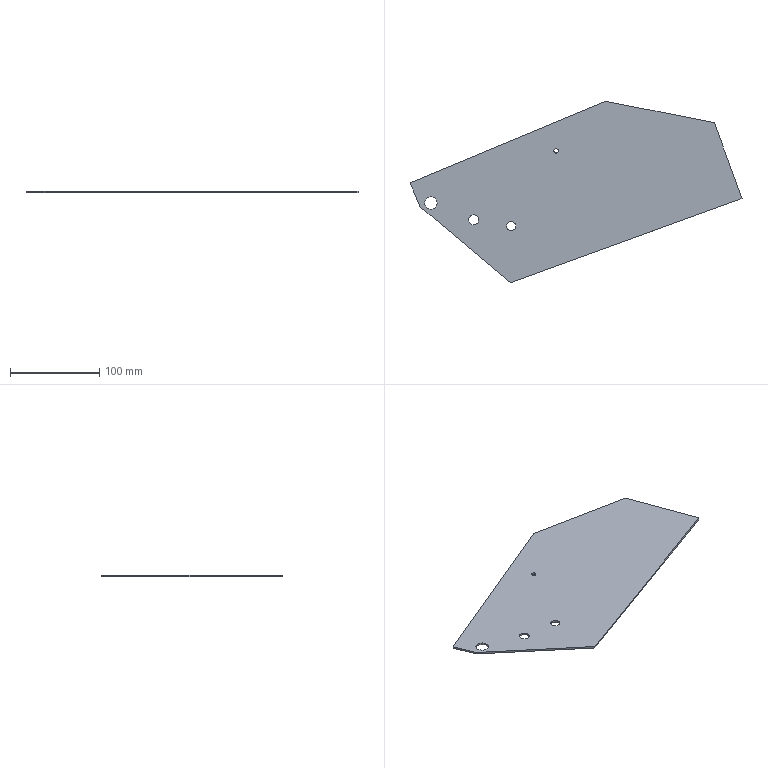Part | SolidWorks | features Cut 6, ICE 4, Extrusion 1, Fillet 1 | 1 solid | 16 faces | box 372.459 x 203.626 x 2 mm | volume 88439 mm3 | cylinder 8 | plane 8 | commonest cylinder face diameters 5 x2 10 x2 11 x2 14 x2
STEP:
#1=CARTESIAN_POINT('',(95.45,-23.568,2.));
#2=VERTEX_POINT('',#1);
#3=CARTESIAN_POINT('',(85.45,-23.568,2.));
#4=VERTEX_POINT('',#3);
#5=CARTESIAN_POINT('',(90.45,-23.568,2.));
#6=DIRECTION('',(0.,0.,-1.));
#7=DIRECTION('',(-1.,0.,0.));
#8=AXIS2_PLACEMENT_3D('',#5,#6,#7);
#9=CIRCLE('',#8,5.);
#10=EDGE_CURVE('',#2,#4,#9,.T.);
#11=ORIENTED_EDGE('',*,*,#10,.F.);
#12=CARTESIAN_POINT('',(95.45,-23.568,0.));
#13=VERTEX_POINT('',#12);
#14=CARTESIAN_POINT('',(95.45,-23.568,2.));
#15=DIRECTION('',(0.,0.,-1.));
#16=VECTOR('',#15,1000.);
#17=LINE('',#14,#16);
#18=EDGE_CURVE('',#2,#13,#17,.T.);
#19=ORIENTED_EDGE('',*,*,#18,.T.);
#20=CARTESIAN_POINT('',(85.45,-23.568,0.));
#21=VERTEX_POINT('',#20);
#22=CARTESIAN_POINT('',(90.45,-23.568,0.));
#23=DIRECTION('',(0.,0.,-1.));
#24=DIRECTION('',(-1.,0.,0.));
#25=AXIS2_PLACEMENT_3D('',#22,#23,#24);
#26=CIRCLE('',#25,5.);
#27=EDGE_CURVE('',#13,#21,#26,.T.);
#28=ORIENTED_EDGE('',*,*,#27,.T.);
#29=CARTESIAN_POINT('',(85.45,-23.568,2.));
#30=DIRECTION('',(0.,0.,-1.));
#31=VECTOR('',#30,1000.);
#32=LINE('',#29,#31);
#33=EDGE_CURVE('',#4,#21,#32,.T.);
#34=ORIENTED_EDGE('',*,*,#33,.F.);
#35=EDGE_LOOP('',(#11,#19,#28,#34));
#36=FACE_OUTER_BOUND('',#35,.T.);
#37=CARTESIAN_POINT('',(90.45,-23.568,2.));
#38=DIRECTION('',(0.,0.,-1.));
#39=DIRECTION('',(-1.,0.,0.));
#40=AXIS2_PLACEMENT_3D('',#37,#38,#39);
#41=CYLINDRICAL_SURFACE('',#40,5.);
#42=ADVANCED_FACE('',(#36),#41,.F.);
#43=CARTESIAN_POINT('',(53.907,-16.547,2.));
#44=VERTEX_POINT('',#43);
#45=CARTESIAN_POINT('',(42.907,-16.547,2.));
#46=VERTEX_POINT('',#45);
#47=CARTESIAN_POINT('',(48.407,-16.547,2.));
#48=DIRECTION('',(0.,0.,-1.));
#49=DIRECTION('',(-1.,0.,0.));
#50=AXIS2_PLACEMENT_3D('',#47,#48,#49);
#51=CIRCLE('',#50,5.5);
#52=EDGE_CURVE('',#44,#46,#51,.T.);
#53=ORIENTED_EDGE('',*,*,#52,.F.);
#54=CARTESIAN_POINT('',(53.907,-16.547,0.));
#55=VERTEX_POINT('',#54);
#56=CARTESIAN_POINT('',(53.907,-16.547,2.));
#57=DIRECTION('',(0.,0.,-1.));
#58=VECTOR('',#57,1000.);
#59=LINE('',#56,#58);
#60=EDGE_CURVE('',#44,#55,#59,.T.);
#61=ORIENTED_EDGE('',*,*,#60,.T.);
#62=CARTESIAN_POINT('',(42.907,-16.547,0.));
#63=VERTEX_POINT('',#62);
#64=CARTESIAN_POINT('',(48.407,-16.547,0.));
#65=DIRECTION('',(0.,0.,-1.));
#66=DIRECTION('',(-1.,0.,0.));
#67=AXIS2_PLACEMENT_3D('',#64,#65,#66);
#68=CIRCLE('',#67,5.5);
#69=EDGE_CURVE('',#55,#63,#68,.T.);
#70=ORIENTED_EDGE('',*,*,#69,.T.);
#71=CARTESIAN_POINT('',(42.907,-16.547,2.));
#72=DIRECTION('',(0.,0.,-1.));
#73=VECTOR('',#72,1000.);
#74=LINE('',#71,#73);
#75=EDGE_CURVE('',#46,#63,#74,.T.);
#76=ORIENTED_EDGE('',*,*,#75,.F.);
#77=EDGE_LOOP('',(#53,#61,#70,#76));
#78=FACE_OUTER_BOUND('',#77,.T.);
#79=CARTESIAN_POINT('',(48.407,-16.547,2.));
#80=DIRECTION('',(0.,0.,-1.));
#81=DIRECTION('',(-1.,0.,0.));
#82=AXIS2_PLACEMENT_3D('',#79,#80,#81);
#83=CYLINDRICAL_SURFACE('',#82,5.5);
#84=ADVANCED_FACE('',(#78),#83,.F.);
#85=CARTESIAN_POINT('',(138.278,60.764,0.));
#86=VERTEX_POINT('',#85);
#87=CARTESIAN_POINT('',(143.278,60.764,0.));
#88=VERTEX_POINT('',#87);
#89=CARTESIAN_POINT('',(140.778,60.764,0.));
#90=DIRECTION('',(0.,0.,1.));
#91=DIRECTION('',(1.,0.,0.));
#92=AXIS2_PLACEMENT_3D('',#89,#90,#91);
#93=CIRCLE('',#92,2.5);
#94=EDGE_CURVE('',#86,#88,#93,.T.);
#95=ORIENTED_EDGE('',*,*,#94,.F.);
#96=CARTESIAN_POINT('',(138.278,60.764,2.));
#97=VERTEX_POINT('',#96);
#98=CARTESIAN_POINT('',(138.278,60.764,0.));
#99=DIRECTION('',(0.,0.,1.));
#100=VECTOR('',#99,1000.);
#101=LINE('',#98,#100);
#102=EDGE_CURVE('',#86,#97,#101,.T.);
#103=ORIENTED_EDGE('',*,*,#102,.T.);
#104=CARTESIAN_POINT('',(143.278,60.764,2.));
#105=VERTEX_POINT('',#104);
#106=CARTESIAN_POINT('',(140.778,60.764,2.));
#107=DIRECTION('',(0.,0.,1.));
#108=DIRECTION('',(1.,0.,0.));
#109=AXIS2_PLACEMENT_3D('',#106,#107,#108);
#110=CIRCLE('',#109,2.5);
#111=EDGE_CURVE('',#97,#105,#110,.T.);
#112=ORIENTED_EDGE('',*,*,#111,.T.);
#113=CARTESIAN_POINT('',(143.278,60.764,0.));
#114=DIRECTION('',(0.,0.,1.));
#115=VECTOR('',#114,1000.);
#116=LINE('',#113,#115);
#117=EDGE_CURVE('',#88,#105,#116,.T.);
#118=ORIENTED_EDGE('',*,*,#117,.F.);
#119=EDGE_LOOP('',(#95,#103,#112,#118));
#120=FACE_OUTER_BOUND('',#119,.T.);
#121=CARTESIAN_POINT('',(140.778,60.764,0.));
#122=DIRECTION('',(0.,0.,1.));
#123=DIRECTION('',(1.,0.,0.));
#124=AXIS2_PLACEMENT_3D('',#121,#122,#123);
#125=CYLINDRICAL_SURFACE('',#124,2.5);
#126=ADVANCED_FACE('',(#120),#125,.F.);
#127=CARTESIAN_POINT('',(-6.599,2.274,2.));
#128=VERTEX_POINT('',#127);
#129=CARTESIAN_POINT('',(7.401,2.274,2.));
#130=VERTEX_POINT('',#129);
#131=CARTESIAN_POINT('',(0.401,2.274,2.));
#132=DIRECTION('',(0.,0.,1.));
#133=DIRECTION('',(1.,0.,0.));
#134=AXIS2_PLACEMENT_3D('',#131,#132,#133);
#135=CIRCLE('',#134,7.);
#136=EDGE_CURVE('',#128,#130,#135,.T.);
#137=ORIENTED_EDGE('',*,*,#136,.T.);
#138=CARTESIAN_POINT('',(7.401,2.274,0.));
#139=VERTEX_POINT('',#138);
#140=CARTESIAN_POINT('',(7.401,2.274,16.));
#141=DIRECTION('',(0.,0.,-1.));
#142=VECTOR('',#141,1000.);
#143=LINE('',#140,#142);
#144=EDGE_CURVE('',#130,#139,#143,.T.);
#145=ORIENTED_EDGE('',*,*,#144,.T.);
#146=CARTESIAN_POINT('',(-6.599,2.274,0.));
#147=VERTEX_POINT('',#146);
#148=CARTESIAN_POINT('',(0.401,2.274,0.));
#149=DIRECTION('',(0.,0.,-1.));
#150=DIRECTION('',(-1.,0.,0.));
#151=AXIS2_PLACEMENT_3D('',#148,#149,#150);
#152=CIRCLE('',#151,7.);
#153=EDGE_CURVE('',#139,#147,#152,.T.);
#154=ORIENTED_EDGE('',*,*,#153,.T.);
#155=CARTESIAN_POINT('',(-6.599,2.274,16.));
#156=DIRECTION('',(0.,0.,-1.));
#157=VECTOR('',#156,1000.);
#158=LINE('',#155,#157);
#159=EDGE_CURVE('',#128,#147,#158,.T.);
#160=ORIENTED_EDGE('',*,*,#159,.F.);
#161=EDGE_LOOP('',(#137,#145,#154,#160));
#162=FACE_OUTER_BOUND('',#161,.T.);
#163=CARTESIAN_POINT('',(0.401,2.274,16.));
#164=DIRECTION('',(0.,0.,-1.));
#165=DIRECTION('',(-1.,0.,0.));
#166=AXIS2_PLACEMENT_3D('',#163,#164,#165);
#167=CYLINDRICAL_SURFACE('',#166,7.);
#168=ADVANCED_FACE('',(#162),#167,.F.);
#169=CARTESIAN_POINT('',(90.45,-23.568,2.));
#170=DIRECTION('',(0.,0.,-1.));
#171=DIRECTION('',(-1.,0.,0.));
#172=AXIS2_PLACEMENT_3D('',#169,#170,#171);
#173=CIRCLE('',#172,5.);
#174=EDGE_CURVE('',#4,#2,#173,.T.);
#175=ORIENTED_EDGE('',*,*,#174,.T.);
#176=ORIENTED_EDGE('',*,*,#10,.T.);
#177=EDGE_LOOP('',(#175,#176));
#178=FACE_BOUND('',#177,.T.);
#179=CARTESIAN_POINT('',(48.407,-16.547,2.));
#180=DIRECTION('',(0.,0.,-1.));
#181=DIRECTION('',(-1.,0.,0.));
#182=AXIS2_PLACEMENT_3D('',#179,#180,#181);
#183=CIRCLE('',#182,5.5);
#184=EDGE_CURVE('',#46,#44,#183,.T.);
#185=ORIENTED_EDGE('',*,*,#184,.T.);
#186=ORIENTED_EDGE('',*,*,#52,.T.);
#187=EDGE_LOOP('',(#185,#186));
#188=FACE_BOUND('',#187,.T.);
#189=CARTESIAN_POINT('',(140.778,60.764,2.));
#190=DIRECTION('',(0.,0.,1.));
#191=DIRECTION('',(1.,0.,0.));
#192=AXIS2_PLACEMENT_3D('',#189,#190,#191);
#193=CIRCLE('',#192,2.5);
#194=EDGE_CURVE('',#105,#97,#193,.T.);
#195=ORIENTED_EDGE('',*,*,#194,.F.);
#196=ORIENTED_EDGE('',*,*,#111,.F.);
#197=EDGE_LOOP('',(#195,#196));
#198=FACE_BOUND('',#197,.T.);
#199=CARTESIAN_POINT('',(-11.929,-1.739,2.));
#200=VERTEX_POINT('',#199);
#201=CARTESIAN_POINT('',(-23.068,24.995,2.));
#202=VERTEX_POINT('',#201);
#203=CARTESIAN_POINT('',(35.106,-114.625,2.));
#204=DIRECTION('',(-0.3846,0.9231,0.));
#205=VECTOR('',#204,1000.);
#206=LINE('',#203,#205);
#207=EDGE_CURVE('',#200,#202,#206,.T.);
#208=ORIENTED_EDGE('',*,*,#207,.F.);
#209=CARTESIAN_POINT('',(89.89,-87.176,2.));
#210=VERTEX_POINT('',#209);
#211=CARTESIAN_POINT('',(-5.785,-6.894,2.));
#212=DIRECTION('',(0.766,-0.6428,0.));
#213=VECTOR('',#212,1000.);
#214=LINE('',#211,#213);
#215=EDGE_CURVE('',#200,#210,#214,.T.);
#216=ORIENTED_EDGE('',*,*,#215,.T.);
#217=CARTESIAN_POINT('',(349.391,7.275,2.));
#218=VERTEX_POINT('',#217);
#219=CARTESIAN_POINT('',(362.494,12.044,2.));
#220=DIRECTION('',(0.9397,0.342,0.));
#221=VECTOR('',#220,1000.);
#222=LINE('',#219,#221);
#223=EDGE_CURVE('',#210,#218,#222,.T.);
#224=ORIENTED_EDGE('',*,*,#223,.T.);
#225=CARTESIAN_POINT('',(318.426,92.35,2.));
#226=VERTEX_POINT('',#225);
#227=CARTESIAN_POINT('',(348.707,9.154,2.));
#228=DIRECTION('',(0.342,-0.9397,0.));
#229=VECTOR('',#228,1000.);
#230=LINE('',#227,#229);
#231=EDGE_CURVE('',#226,#218,#230,.T.);
#232=ORIENTED_EDGE('',*,*,#231,.F.);
#233=CARTESIAN_POINT('',(196.426,116.45,2.));
#234=VERTEX_POINT('',#233);
#235=CARTESIAN_POINT('',(318.426,92.35,2.));
#236=DIRECTION('',(0.981,-0.1938,0.));
#237=VECTOR('',#236,1000.);
#238=LINE('',#235,#237);
#239=EDGE_CURVE('',#234,#226,#238,.T.);
#240=ORIENTED_EDGE('',*,*,#239,.F.);
#241=CARTESIAN_POINT('',(92.709,73.235,2.));
#242=DIRECTION('',(0.9231,0.3846,0.));
#243=VECTOR('',#242,1000.);
#244=LINE('',#241,#243);
#245=EDGE_CURVE('',#202,#234,#244,.T.);
#246=ORIENTED_EDGE('',*,*,#245,.F.);
#247=EDGE_LOOP('',(#208,#216,#224,#232,#240,#246));
#248=FACE_OUTER_BOUND('',#247,.T.);
#249=ORIENTED_EDGE('',*,*,#136,.F.);
#250=CARTESIAN_POINT('',(0.401,2.274,2.));
#251=DIRECTION('',(0.,0.,1.));
#252=DIRECTION('',(1.,0.,0.));
#253=AXIS2_PLACEMENT_3D('',#250,#251,#252);
#254=CIRCLE('',#253,7.);
#255=EDGE_CURVE('',#130,#128,#254,.T.);
#256=ORIENTED_EDGE('',*,*,#255,.F.);
#257=EDGE_LOOP('',(#249,#256));
#258=FACE_BOUND('',#257,.T.);
#259=CARTESIAN_POINT('',(359.416,20.501,2.));
#260=DIRECTION('',(0.,0.,1.));
#261=DIRECTION('',(1.,0.,0.));
#262=AXIS2_PLACEMENT_3D('',#259,#260,#261);
#263=PLANE('',#262);
#264=ADVANCED_FACE('',(#178,#188,#198,#248,#258),#263,.T.);
#265=CARTESIAN_POINT('',(90.45,-23.568,0.));
#266=DIRECTION('',(0.,0.,-1.));
#267=DIRECTION('',(-1.,0.,0.));
#268=AXIS2_PLACEMENT_3D('',#265,#266,#267);
#269=CIRCLE('',#268,5.);
#270=EDGE_CURVE('',#21,#13,#269,.T.);
#271=ORIENTED_EDGE('',*,*,#270,.F.);
#272=ORIENTED_EDGE('',*,*,#27,.F.);
#273=EDGE_LOOP('',(#271,#272));
#274=FACE_BOUND('',#273,.T.);
#275=CARTESIAN_POINT('',(48.407,-16.547,0.));
#276=DIRECTION('',(0.,0.,-1.));
#277=DIRECTION('',(-1.,0.,0.));
#278=AXIS2_PLACEMENT_3D('',#275,#276,#277);
#279=CIRCLE('',#278,5.5);
#280=EDGE_CURVE('',#63,#55,#279,.T.);
#281=ORIENTED_EDGE('',*,*,#280,.F.);
#282=ORIENTED_EDGE('',*,*,#69,.F.);
#283=EDGE_LOOP('',(#281,#282));
#284=FACE_BOUND('',#283,.T.);
#285=CARTESIAN_POINT('',(140.778,60.764,0.));
#286=DIRECTION('',(0.,0.,1.));
#287=DIRECTION('',(1.,0.,0.));
#288=AXIS2_PLACEMENT_3D('',#285,#286,#287);
#289=CIRCLE('',#288,2.5);
#290=EDGE_CURVE('',#88,#86,#289,.T.);
#291=ORIENTED_EDGE('',*,*,#290,.T.);
#292=ORIENTED_EDGE('',*,*,#94,.T.);
#293=EDGE_LOOP('',(#291,#292));
#294=FACE_BOUND('',#293,.T.);
#295=CARTESIAN_POINT('',(0.401,2.274,0.));
#296=DIRECTION('',(0.,0.,-1.));
#297=DIRECTION('',(-1.,0.,0.));
#298=AXIS2_PLACEMENT_3D('',#295,#296,#297);
#299=CIRCLE('',#298,7.);
#300=EDGE_CURVE('',#147,#139,#299,.T.);
#301=ORIENTED_EDGE('',*,*,#300,.F.);
#302=ORIENTED_EDGE('',*,*,#153,.F.);
#303=EDGE_LOOP('',(#301,#302));
#304=FACE_BOUND('',#303,.T.);
#305=CARTESIAN_POINT('',(-11.929,-1.739,0.));
#306=VERTEX_POINT('',#305);
#307=CARTESIAN_POINT('',(89.89,-87.176,0.));
#308=VERTEX_POINT('',#307);
#309=CARTESIAN_POINT('',(-5.785,-6.894,0.));
#310=DIRECTION('',(0.766,-0.6428,0.));
#311=VECTOR('',#310,1000.);
#312=LINE('',#309,#311);
#313=EDGE_CURVE('',#306,#308,#312,.T.);
#314=ORIENTED_EDGE('',*,*,#313,.F.);
#315=CARTESIAN_POINT('',(-23.068,24.995,0.));
#316=VERTEX_POINT('',#315);
#317=CARTESIAN_POINT('',(-23.068,24.995,0.));
#318=DIRECTION('',(0.3846,-0.9231,0.));
#319=VECTOR('',#318,1000.);
#320=LINE('',#317,#319);
#321=EDGE_CURVE('',#316,#306,#320,.T.);
#322=ORIENTED_EDGE('',*,*,#321,.F.);
#323=CARTESIAN_POINT('',(196.426,116.45,0.));
#324=VERTEX_POINT('',#323);
#325=CARTESIAN_POINT('',(283.449,152.709,0.));
#326=DIRECTION('',(0.9231,0.3846,0.));
#327=VECTOR('',#326,1000.);
#328=LINE('',#325,#327);
#329=EDGE_CURVE('',#316,#324,#328,.T.);
#330=ORIENTED_EDGE('',*,*,#329,.T.);
#331=CARTESIAN_POINT('',(318.426,92.35,0.));
#332=VERTEX_POINT('',#331);
#333=CARTESIAN_POINT('',(371.536,81.858,0.));
#334=DIRECTION('',(0.981,-0.1938,0.));
#335=VECTOR('',#334,1000.);
#336=LINE('',#333,#335);
#337=EDGE_CURVE('',#324,#332,#336,.T.);
#338=ORIENTED_EDGE('',*,*,#337,.T.);
#339=CARTESIAN_POINT('',(349.391,7.275,0.));
#340=VERTEX_POINT('',#339);
#341=CARTESIAN_POINT('',(349.391,7.275,0.));
#342=DIRECTION('',(0.342,-0.9397,0.));
#343=VECTOR('',#342,1000.);
#344=LINE('',#341,#343);
#345=EDGE_CURVE('',#332,#340,#344,.T.);
#346=ORIENTED_EDGE('',*,*,#345,.T.);
#347=CARTESIAN_POINT('',(362.494,12.044,0.));
#348=DIRECTION('',(0.9397,0.342,0.));
#349=VECTOR('',#348,1000.);
#350=LINE('',#347,#349);
#351=EDGE_CURVE('',#308,#340,#350,.T.);
#352=ORIENTED_EDGE('',*,*,#351,.F.);
#353=EDGE_LOOP('',(#314,#322,#330,#338,#346,#352));
#354=FACE_OUTER_BOUND('',#353,.T.);
#355=CARTESIAN_POINT('',(359.416,20.501,0.));
#356=DIRECTION('',(0.,0.,1.));
#357=DIRECTION('',(1.,0.,0.));
#358=AXIS2_PLACEMENT_3D('',#355,#356,#357);
#359=PLANE('',#358);
#360=ADVANCED_FACE('',(#274,#284,#294,#304,#354),#359,.F.);
#361=ORIENTED_EDGE('',*,*,#215,.F.);
#362=CARTESIAN_POINT('',(-11.929,-1.739,10.));
#363=DIRECTION('',(0.,0.,-1.));
#364=VECTOR('',#363,1000.);
#365=LINE('',#362,#364);
#366=EDGE_CURVE('',#200,#306,#365,.T.);
#367=ORIENTED_EDGE('',*,*,#366,.T.);
#368=ORIENTED_EDGE('',*,*,#313,.T.);
#369=CARTESIAN_POINT('',(89.89,-87.176,2.));
#370=DIRECTION('',(0.,0.,-1.));
#371=VECTOR('',#370,1000.);
#372=LINE('',#369,#371);
#373=EDGE_CURVE('',#210,#308,#372,.T.);
#374=ORIENTED_EDGE('',*,*,#373,.F.);
#375=EDGE_LOOP('',(#361,#367,#368,#374));
#376=FACE_OUTER_BOUND('',#375,.T.);
#377=CARTESIAN_POINT('',(-5.785,-6.894,2.));
#378=DIRECTION('',(0.6428,0.766,0.));
#379=DIRECTION('',(-0.766,0.6428,0.));
#380=AXIS2_PLACEMENT_3D('',#377,#378,#379);
#381=PLANE('',#380);
#382=ADVANCED_FACE('',(#376),#381,.F.);
#383=ORIENTED_EDGE('',*,*,#351,.T.);
#384=CARTESIAN_POINT('',(349.391,7.275,2.));
#385=DIRECTION('',(0.,0.,-1.));
#386=VECTOR('',#385,1000.);
#387=LINE('',#384,#386);
#388=EDGE_CURVE('',#218,#340,#387,.T.);
#389=ORIENTED_EDGE('',*,*,#388,.F.);
#390=ORIENTED_EDGE('',*,*,#223,.F.);
#391=ORIENTED_EDGE('',*,*,#373,.T.);
#392=EDGE_LOOP('',(#383,#389,#390,#391));
#393=FACE_OUTER_BOUND('',#392,.T.);
#394=CARTESIAN_POINT('',(362.494,12.044,2.));
#395=DIRECTION('',(-0.342,0.9397,0.));
#396=DIRECTION('',(-0.9397,-0.342,0.));
#397=AXIS2_PLACEMENT_3D('',#394,#395,#396);
#398=PLANE('',#397);
#399=ADVANCED_FACE('',(#393),#398,.F.);
#400=CARTESIAN_POINT('',(-23.068,24.995,2.));
#401=DIRECTION('',(0.,0.,-1.));
#402=VECTOR('',#401,1000.);
#403=LINE('',#400,#402);
#404=EDGE_CURVE('',#202,#316,#403,.T.);
#405=ORIENTED_EDGE('',*,*,#404,.F.);
#406=ORIENTED_EDGE('',*,*,#245,.T.);
#407=CARTESIAN_POINT('',(196.426,116.45,-8.));
#408=DIRECTION('',(0.,0.,1.));
#409=VECTOR('',#408,1000.);
#410=LINE('',#407,#409);
#411=EDGE_CURVE('',#324,#234,#410,.T.);
#412=ORIENTED_EDGE('',*,*,#411,.F.);
#413=ORIENTED_EDGE('',*,*,#329,.F.);
#414=EDGE_LOOP('',(#405,#406,#412,#413));
#415=FACE_OUTER_BOUND('',#414,.T.);
#416=CARTESIAN_POINT('',(283.449,152.709,2.));
#417=DIRECTION('',(-0.3846,0.9231,0.));
#418=DIRECTION('',(-0.9231,-0.3846,0.));
#419=AXIS2_PLACEMENT_3D('',#416,#417,#418);
#420=PLANE('',#419);
#421=ADVANCED_FACE('',(#415),#420,.T.);
#422=ORIENTED_EDGE('',*,*,#144,.F.);
#423=ORIENTED_EDGE('',*,*,#255,.T.);
#424=ORIENTED_EDGE('',*,*,#159,.T.);
#425=ORIENTED_EDGE('',*,*,#300,.T.);
#426=EDGE_LOOP('',(#422,#423,#424,#425));
#427=FACE_OUTER_BOUND('',#426,.T.);
#428=CARTESIAN_POINT('',(0.401,2.274,16.));
#429=DIRECTION('',(0.,0.,-1.));
#430=DIRECTION('',(-1.,0.,0.));
#431=AXIS2_PLACEMENT_3D('',#428,#429,#430);
#432=CYLINDRICAL_SURFACE('',#431,7.);
#433=ADVANCED_FACE('',(#427),#432,.F.);
#434=CARTESIAN_POINT('',(318.426,92.35,2.));
#435=DIRECTION('',(0.,0.,-1.));
#436=VECTOR('',#435,1000.);
#437=LINE('',#434,#436);
#438=EDGE_CURVE('',#226,#332,#437,.T.);
#439=ORIENTED_EDGE('',*,*,#438,.F.);
#440=ORIENTED_EDGE('',*,*,#231,.T.);
#441=ORIENTED_EDGE('',*,*,#388,.T.);
#442=ORIENTED_EDGE('',*,*,#345,.F.);
#443=EDGE_LOOP('',(#439,#440,#441,#442));
#444=FACE_OUTER_BOUND('',#443,.T.);
#445=CARTESIAN_POINT('',(349.391,7.275,2.));
#446=DIRECTION('',(0.9397,0.342,0.));
#447=DIRECTION('',(-0.342,0.9397,0.));
#448=AXIS2_PLACEMENT_3D('',#445,#446,#447);
#449=PLANE('',#448);
#450=ADVANCED_FACE('',(#444),#449,.T.);
#451=ORIENTED_EDGE('',*,*,#411,.T.);
#452=ORIENTED_EDGE('',*,*,#239,.T.);
#453=ORIENTED_EDGE('',*,*,#438,.T.);
#454=ORIENTED_EDGE('',*,*,#337,.F.);
#455=EDGE_LOOP('',(#451,#452,#453,#454));
#456=FACE_OUTER_BOUND('',#455,.T.);
#457=CARTESIAN_POINT('',(318.426,92.35,-8.));
#458=DIRECTION('',(-0.1938,-0.981,0.));
#459=DIRECTION('',(0.981,-0.1938,0.));
#460=AXIS2_PLACEMENT_3D('',#457,#458,#459);
#461=PLANE('',#460);
#462=ADVANCED_FACE('',(#456),#461,.F.);
#463=ORIENTED_EDGE('',*,*,#207,.T.);
#464=ORIENTED_EDGE('',*,*,#404,.T.);
#465=ORIENTED_EDGE('',*,*,#321,.T.);
#466=ORIENTED_EDGE('',*,*,#366,.F.);
#467=EDGE_LOOP('',(#463,#464,#465,#466));
#468=FACE_OUTER_BOUND('',#467,.T.);
#469=CARTESIAN_POINT('',(-23.068,24.995,10.));
#470=DIRECTION('',(0.9231,0.3846,0.));
#471=DIRECTION('',(-0.3846,0.9231,0.));
#472=AXIS2_PLACEMENT_3D('',#469,#470,#471);
#473=PLANE('',#472);
#474=ADVANCED_FACE('',(#468),#473,.F.);
#475=ORIENTED_EDGE('',*,*,#102,.F.);
#476=ORIENTED_EDGE('',*,*,#290,.F.);
#477=ORIENTED_EDGE('',*,*,#117,.T.);
#478=ORIENTED_EDGE('',*,*,#194,.T.);
#479=EDGE_LOOP('',(#475,#476,#477,#478));
#480=FACE_OUTER_BOUND('',#479,.T.);
#481=CARTESIAN_POINT('',(140.778,60.764,0.));
#482=DIRECTION('',(0.,0.,1.));
#483=DIRECTION('',(1.,0.,0.));
#484=AXIS2_PLACEMENT_3D('',#481,#482,#483);
#485=CYLINDRICAL_SURFACE('',#484,2.5);
#486=ADVANCED_FACE('',(#480),#485,.F.);
#487=ORIENTED_EDGE('',*,*,#60,.F.);
#488=ORIENTED_EDGE('',*,*,#184,.F.);
#489=ORIENTED_EDGE('',*,*,#75,.T.);
#490=ORIENTED_EDGE('',*,*,#280,.T.);
#491=EDGE_LOOP('',(#487,#488,#489,#490));
#492=FACE_OUTER_BOUND('',#491,.T.);
#493=CARTESIAN_POINT('',(48.407,-16.547,2.));
#494=DIRECTION('',(0.,0.,-1.));
#495=DIRECTION('',(-1.,0.,0.));
#496=AXIS2_PLACEMENT_3D('',#493,#494,#495);
#497=CYLINDRICAL_SURFACE('',#496,5.5);
#498=ADVANCED_FACE('',(#492),#497,.F.);
#499=ORIENTED_EDGE('',*,*,#18,.F.);
#500=ORIENTED_EDGE('',*,*,#174,.F.);
#501=ORIENTED_EDGE('',*,*,#33,.T.);
#502=ORIENTED_EDGE('',*,*,#270,.T.);
#503=EDGE_LOOP('',(#499,#500,#501,#502));
#504=FACE_OUTER_BOUND('',#503,.T.);
#505=CARTESIAN_POINT('',(90.45,-23.568,2.));
#506=DIRECTION('',(0.,0.,-1.));
#507=DIRECTION('',(-1.,0.,0.));
#508=AXIS2_PLACEMENT_3D('',#505,#506,#507);
#509=CYLINDRICAL_SURFACE('',#508,5.);
#510=ADVANCED_FACE('',(#504),#509,.F.);
#511=CLOSED_SHELL('',(#42,#84,#126,#168,#264,#360,#382,#399,#421,#433,#450,#462,#474,#486,#498,#510));
#512=MANIFOLD_SOLID_BREP('',#511);
#513=CARTESIAN_POINT('',(0.,0.,0.));
#514=DIRECTION('',(0.,0.,1.));
#515=DIRECTION('',(1.,0.,0.));
#516=AXIS2_PLACEMENT_3D('',#513,#514,#515);
#517=(LENGTH_UNIT()NAMED_UNIT(*)SI_UNIT(.MILLI.,.METRE.));
#518=UNCERTAINTY_MEASURE_WITH_UNIT(LENGTH_MEASURE(0.00001),#517,'','');
#519=(NAMED_UNIT(*)PLANE_ANGLE_UNIT()SI_UNIT($,.RADIAN.));
#520=(NAMED_UNIT(*)SI_UNIT($,.STERADIAN.)SOLID_ANGLE_UNIT());
#521=(GEOMETRIC_REPRESENTATION_CONTEXT(3)GLOBAL_UNCERTAINTY_ASSIGNED_CONTEXT((#518))GLOBAL_UNIT_ASSIGNED_CONTEXT((#517,#519,#520))REPRESENTATION_CONTEXT('',''));
#522=ADVANCED_BREP_SHAPE_REPRESENTATION('',(#512,#516),#521);